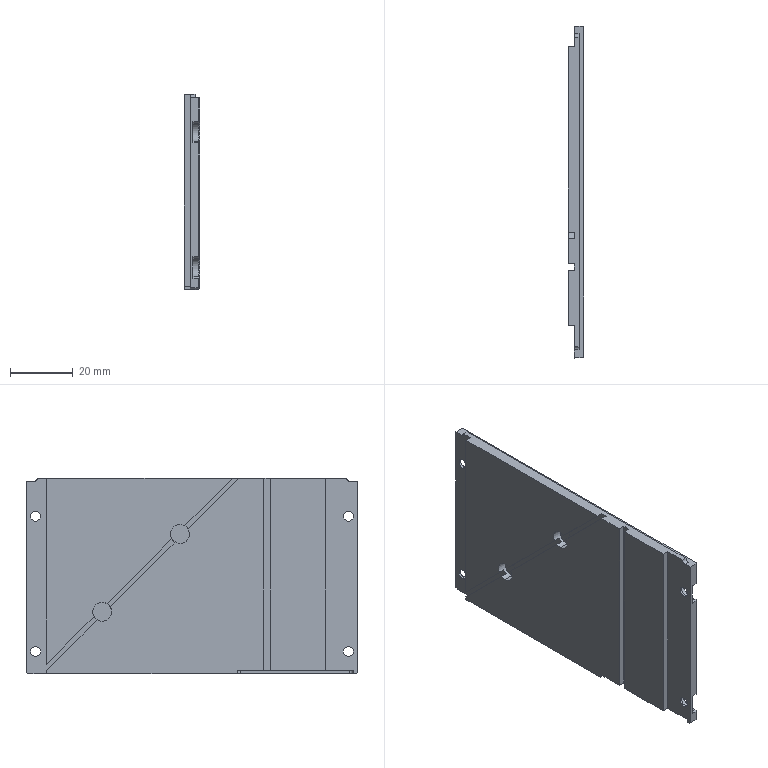Part | SolidWorks | features BaseBody 1 | 1 solid | 126 faces | box 5 x 105.4 x 62 mm | volume 29184 mm3 | plane 74 | cylinder 30 | cone 22 | commonest cylinder face diameters 3.2 x8 3.5 x8 2 x4 5.8 x4 6 x4 1.6 x2